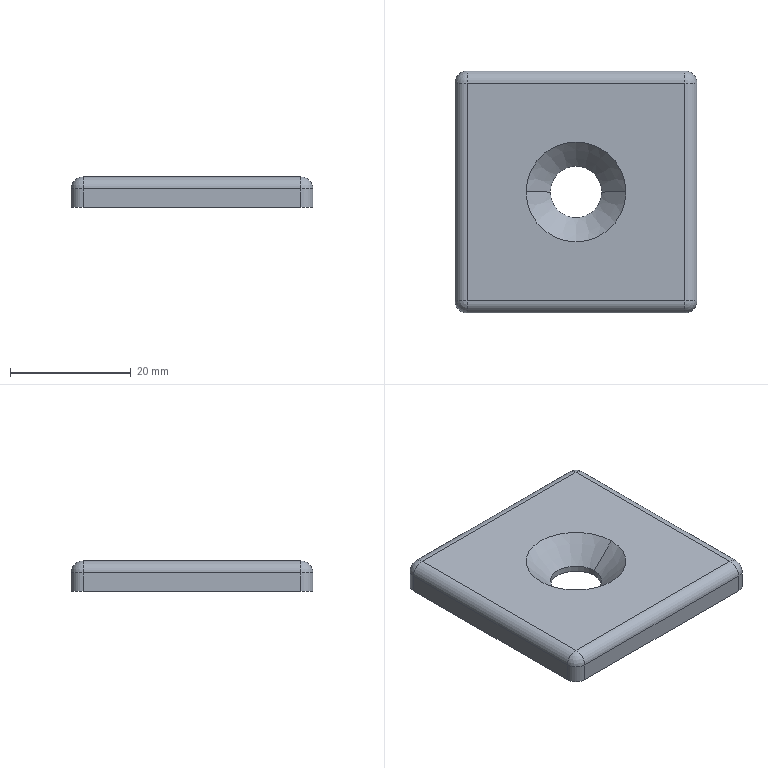Part | NX | features BREP 1 | 1 solid | 22 faces | box 40 x 40 x 5 mm | volume 7286 mm3 | cylinder 10 | plane 6 | sphere 4 | cone 2 | commonest cylinder face diameters 4 x8 8.5 x2
STEP:
#1=CARTESIAN_POINT('',(-4.25,0.,1.));
#2=VERTEX_POINT('',#1);
#3=CARTESIAN_POINT('',(4.25,0.,1.));
#4=VERTEX_POINT('',#3);
#5=CARTESIAN_POINT('',(0.,0.,1.));
#6=DIRECTION('',(0.,0.,1.));
#7=DIRECTION('',(-1.,0.,0.));
#8=AXIS2_PLACEMENT_3D('',#5,#6,#7);
#9=CIRCLE('',#8,4.25);
#10=EDGE_CURVE('',#2,#4,#9,.T.);
#11=ORIENTED_EDGE('',*,*,#10,.F.);
#12=CARTESIAN_POINT('',(-8.25,0.,5.));
#13=VERTEX_POINT('',#12);
#14=CARTESIAN_POINT('',(-4.25,0.,1.));
#15=DIRECTION('',(-0.7071,0.,0.7071));
#16=VECTOR('',#15,1000.);
#17=LINE('',#14,#16);
#18=EDGE_CURVE('',#13,#2,#17,.F.);
#19=ORIENTED_EDGE('',*,*,#18,.F.);
#20=CARTESIAN_POINT('',(8.25,0.,5.));
#21=VERTEX_POINT('',#20);
#22=CARTESIAN_POINT('',(0.,0.,5.));
#23=DIRECTION('',(0.,0.,-1.));
#24=DIRECTION('',(-1.,0.,0.));
#25=AXIS2_PLACEMENT_3D('',#22,#23,#24);
#26=CIRCLE('',#25,8.25);
#27=EDGE_CURVE('',#21,#13,#26,.T.);
#28=ORIENTED_EDGE('',*,*,#27,.F.);
#29=CARTESIAN_POINT('',(4.25,0.,1.));
#30=DIRECTION('',(0.7071,0.,0.7071));
#31=VECTOR('',#30,1000.);
#32=LINE('',#29,#31);
#33=EDGE_CURVE('',#21,#4,#32,.F.);
#34=ORIENTED_EDGE('',*,*,#33,.T.);
#35=EDGE_LOOP('',(#11,#19,#28,#34));
#36=FACE_BOUND('',#35,.T.);
#37=CARTESIAN_POINT('',(0.,0.,1.));
#38=DIRECTION('',(0.,0.,1.));
#39=DIRECTION('',(1.,0.,0.));
#40=AXIS2_PLACEMENT_3D('',#37,#38,#39);
#41=CONICAL_SURFACE('',#40,4.25,0.7854);
#42=ADVANCED_FACE('',(#36),#41,.F.);
#43=CARTESIAN_POINT('',(-4.25,0.,0.));
#44=VERTEX_POINT('',#43);
#45=CARTESIAN_POINT('',(4.25,0.,0.));
#46=VERTEX_POINT('',#45);
#47=CARTESIAN_POINT('',(0.,0.,0.));
#48=DIRECTION('',(0.,0.,1.));
#49=DIRECTION('',(1.,0.,0.));
#50=AXIS2_PLACEMENT_3D('',#47,#48,#49);
#51=CIRCLE('',#50,4.25);
#52=EDGE_CURVE('',#44,#46,#51,.T.);
#53=ORIENTED_EDGE('',*,*,#52,.F.);
#54=CARTESIAN_POINT('',(-4.25,0.,0.));
#55=DIRECTION('',(0.,0.,1.));
#56=VECTOR('',#55,1000.);
#57=LINE('',#54,#56);
#58=EDGE_CURVE('',#2,#44,#57,.F.);
#59=ORIENTED_EDGE('',*,*,#58,.F.);
#60=ORIENTED_EDGE('',*,*,#10,.T.);
#61=CARTESIAN_POINT('',(4.25,0.,0.));
#62=DIRECTION('',(0.,0.,1.));
#63=VECTOR('',#62,1000.);
#64=LINE('',#61,#63);
#65=EDGE_CURVE('',#4,#46,#64,.F.);
#66=ORIENTED_EDGE('',*,*,#65,.T.);
#67=EDGE_LOOP('',(#53,#59,#60,#66));
#68=FACE_BOUND('',#67,.T.);
#69=CARTESIAN_POINT('',(0.,0.,0.));
#70=DIRECTION('',(0.,0.,1.));
#71=DIRECTION('',(1.,0.,0.));
#72=AXIS2_PLACEMENT_3D('',#69,#70,#71);
#73=CYLINDRICAL_SURFACE('',#72,4.25);
#74=ADVANCED_FACE('',(#68),#73,.F.);
#75=CARTESIAN_POINT('',(20.,-18.,0.));
#76=VERTEX_POINT('',#75);
#77=CARTESIAN_POINT('',(20.,18.,0.));
#78=VERTEX_POINT('',#77);
#79=CARTESIAN_POINT('',(20.,-20.,0.));
#80=DIRECTION('',(0.,1.,0.));
#81=VECTOR('',#80,1000.);
#82=LINE('',#79,#81);
#83=EDGE_CURVE('',#76,#78,#82,.T.);
#84=ORIENTED_EDGE('',*,*,#83,.T.);
#85=CARTESIAN_POINT('',(20.,18.,3.));
#86=VERTEX_POINT('',#85);
#87=CARTESIAN_POINT('',(20.,18.,5.));
#88=DIRECTION('',(0.,0.,1.));
#89=VECTOR('',#88,1000.);
#90=LINE('',#87,#89);
#91=EDGE_CURVE('',#78,#86,#90,.T.);
#92=ORIENTED_EDGE('',*,*,#91,.T.);
#93=CARTESIAN_POINT('',(20.,-18.,3.));
#94=VERTEX_POINT('',#93);
#95=CARTESIAN_POINT('',(20.,-20.,3.));
#96=DIRECTION('',(0.,-1.,0.));
#97=VECTOR('',#96,1000.);
#98=LINE('',#95,#97);
#99=EDGE_CURVE('',#86,#94,#98,.T.);
#100=ORIENTED_EDGE('',*,*,#99,.T.);
#101=CARTESIAN_POINT('',(20.,-18.,5.));
#102=DIRECTION('',(0.,0.,-1.));
#103=VECTOR('',#102,1000.);
#104=LINE('',#101,#103);
#105=EDGE_CURVE('',#94,#76,#104,.T.);
#106=ORIENTED_EDGE('',*,*,#105,.T.);
#107=EDGE_LOOP('',(#84,#92,#100,#106));
#108=FACE_BOUND('',#107,.T.);
#109=CARTESIAN_POINT('',(20.,-20.,5.));
#110=DIRECTION('',(-1.,0.,0.));
#111=DIRECTION('',(0.,0.,1.));
#112=AXIS2_PLACEMENT_3D('',#109,#110,#111);
#113=PLANE('',#112);
#114=ADVANCED_FACE('',(#108),#113,.F.);
#115=CARTESIAN_POINT('',(18.,20.,0.));
#116=VERTEX_POINT('',#115);
#117=CARTESIAN_POINT('',(-18.,20.,0.));
#118=VERTEX_POINT('',#117);
#119=CARTESIAN_POINT('',(-20.,20.,0.));
#120=DIRECTION('',(-1.,0.,0.));
#121=VECTOR('',#120,1000.);
#122=LINE('',#119,#121);
#123=EDGE_CURVE('',#116,#118,#122,.T.);
#124=ORIENTED_EDGE('',*,*,#123,.T.);
#125=CARTESIAN_POINT('',(-18.,20.,3.));
#126=VERTEX_POINT('',#125);
#127=CARTESIAN_POINT('',(-18.,20.,5.));
#128=DIRECTION('',(0.,0.,1.));
#129=VECTOR('',#128,1000.);
#130=LINE('',#127,#129);
#131=EDGE_CURVE('',#118,#126,#130,.T.);
#132=ORIENTED_EDGE('',*,*,#131,.T.);
#133=CARTESIAN_POINT('',(18.,20.,3.));
#134=VERTEX_POINT('',#133);
#135=CARTESIAN_POINT('',(-20.,20.,3.));
#136=DIRECTION('',(1.,0.,0.));
#137=VECTOR('',#136,1000.);
#138=LINE('',#135,#137);
#139=EDGE_CURVE('',#126,#134,#138,.T.);
#140=ORIENTED_EDGE('',*,*,#139,.T.);
#141=CARTESIAN_POINT('',(18.,20.,5.));
#142=DIRECTION('',(0.,0.,-1.));
#143=VECTOR('',#142,1000.);
#144=LINE('',#141,#143);
#145=EDGE_CURVE('',#134,#116,#144,.T.);
#146=ORIENTED_EDGE('',*,*,#145,.T.);
#147=EDGE_LOOP('',(#124,#132,#140,#146));
#148=FACE_BOUND('',#147,.T.);
#149=CARTESIAN_POINT('',(-20.,20.,5.));
#150=DIRECTION('',(0.,-1.,0.));
#151=DIRECTION('',(0.,0.,-1.));
#152=AXIS2_PLACEMENT_3D('',#149,#150,#151);
#153=PLANE('',#152);
#154=ADVANCED_FACE('',(#148),#153,.F.);
#155=CARTESIAN_POINT('',(-20.,-18.,3.));
#156=VERTEX_POINT('',#155);
#157=CARTESIAN_POINT('',(-20.,18.,3.));
#158=VERTEX_POINT('',#157);
#159=CARTESIAN_POINT('',(-20.,-20.,3.));
#160=DIRECTION('',(0.,1.,0.));
#161=VECTOR('',#160,1000.);
#162=LINE('',#159,#161);
#163=EDGE_CURVE('',#156,#158,#162,.T.);
#164=ORIENTED_EDGE('',*,*,#163,.T.);
#165=CARTESIAN_POINT('',(-20.,18.,0.));
#166=VERTEX_POINT('',#165);
#167=CARTESIAN_POINT('',(-20.,18.,5.));
#168=DIRECTION('',(0.,0.,-1.));
#169=VECTOR('',#168,1000.);
#170=LINE('',#167,#169);
#171=EDGE_CURVE('',#158,#166,#170,.T.);
#172=ORIENTED_EDGE('',*,*,#171,.T.);
#173=CARTESIAN_POINT('',(-20.,-18.,0.));
#174=VERTEX_POINT('',#173);
#175=CARTESIAN_POINT('',(-20.,-20.,0.));
#176=DIRECTION('',(0.,-1.,0.));
#177=VECTOR('',#176,1000.);
#178=LINE('',#175,#177);
#179=EDGE_CURVE('',#166,#174,#178,.T.);
#180=ORIENTED_EDGE('',*,*,#179,.T.);
#181=CARTESIAN_POINT('',(-20.,-18.,5.));
#182=DIRECTION('',(0.,0.,1.));
#183=VECTOR('',#182,1000.);
#184=LINE('',#181,#183);
#185=EDGE_CURVE('',#174,#156,#184,.T.);
#186=ORIENTED_EDGE('',*,*,#185,.T.);
#187=EDGE_LOOP('',(#164,#172,#180,#186));
#188=FACE_BOUND('',#187,.T.);
#189=CARTESIAN_POINT('',(-20.,-20.,5.));
#190=DIRECTION('',(1.,0.,0.));
#191=DIRECTION('',(0.,1.,0.));
#192=AXIS2_PLACEMENT_3D('',#189,#190,#191);
#193=PLANE('',#192);
#194=ADVANCED_FACE('',(#188),#193,.F.);
#195=CARTESIAN_POINT('',(-18.,-20.,0.));
#196=VERTEX_POINT('',#195);
#197=CARTESIAN_POINT('',(18.,-20.,0.));
#198=VERTEX_POINT('',#197);
#199=CARTESIAN_POINT('',(-20.,-20.,0.));
#200=DIRECTION('',(1.,0.,0.));
#201=VECTOR('',#200,1000.);
#202=LINE('',#199,#201);
#203=EDGE_CURVE('',#196,#198,#202,.T.);
#204=ORIENTED_EDGE('',*,*,#203,.T.);
#205=CARTESIAN_POINT('',(18.,-20.,3.));
#206=VERTEX_POINT('',#205);
#207=CARTESIAN_POINT('',(18.,-20.,5.));
#208=DIRECTION('',(0.,0.,1.));
#209=VECTOR('',#208,1000.);
#210=LINE('',#207,#209);
#211=EDGE_CURVE('',#198,#206,#210,.T.);
#212=ORIENTED_EDGE('',*,*,#211,.T.);
#213=CARTESIAN_POINT('',(-18.,-20.,3.));
#214=VERTEX_POINT('',#213);
#215=CARTESIAN_POINT('',(-20.,-20.,3.));
#216=DIRECTION('',(-1.,0.,0.));
#217=VECTOR('',#216,1000.);
#218=LINE('',#215,#217);
#219=EDGE_CURVE('',#206,#214,#218,.T.);
#220=ORIENTED_EDGE('',*,*,#219,.T.);
#221=CARTESIAN_POINT('',(-18.,-20.,5.));
#222=DIRECTION('',(0.,0.,-1.));
#223=VECTOR('',#222,1000.);
#224=LINE('',#221,#223);
#225=EDGE_CURVE('',#214,#196,#224,.T.);
#226=ORIENTED_EDGE('',*,*,#225,.T.);
#227=EDGE_LOOP('',(#204,#212,#220,#226));
#228=FACE_BOUND('',#227,.T.);
#229=CARTESIAN_POINT('',(-20.,-20.,5.));
#230=DIRECTION('',(0.,1.,0.));
#231=DIRECTION('',(1.,0.,0.));
#232=AXIS2_PLACEMENT_3D('',#229,#230,#231);
#233=PLANE('',#232);
#234=ADVANCED_FACE('',(#228),#233,.F.);
#235=CARTESIAN_POINT('',(-18.,18.,5.));
#236=VERTEX_POINT('',#235);
#237=CARTESIAN_POINT('',(-18.,-18.,5.));
#238=VERTEX_POINT('',#237);
#239=CARTESIAN_POINT('',(-18.,0.,5.));
#240=DIRECTION('',(0.,-1.,0.));
#241=VECTOR('',#240,1000.);
#242=LINE('',#239,#241);
#243=EDGE_CURVE('',#236,#238,#242,.T.);
#244=ORIENTED_EDGE('',*,*,#243,.T.);
#245=CARTESIAN_POINT('',(18.,-18.,5.));
#246=VERTEX_POINT('',#245);
#247=CARTESIAN_POINT('',(0.,-18.,5.));
#248=DIRECTION('',(1.,0.,0.));
#249=VECTOR('',#248,1000.);
#250=LINE('',#247,#249);
#251=EDGE_CURVE('',#238,#246,#250,.T.);
#252=ORIENTED_EDGE('',*,*,#251,.T.);
#253=CARTESIAN_POINT('',(18.,18.,5.));
#254=VERTEX_POINT('',#253);
#255=CARTESIAN_POINT('',(18.,0.,5.));
#256=DIRECTION('',(0.,1.,0.));
#257=VECTOR('',#256,1000.);
#258=LINE('',#255,#257);
#259=EDGE_CURVE('',#246,#254,#258,.T.);
#260=ORIENTED_EDGE('',*,*,#259,.T.);
#261=CARTESIAN_POINT('',(0.,18.,5.));
#262=DIRECTION('',(-1.,0.,0.));
#263=VECTOR('',#262,1000.);
#264=LINE('',#261,#263);
#265=EDGE_CURVE('',#254,#236,#264,.T.);
#266=ORIENTED_EDGE('',*,*,#265,.T.);
#267=EDGE_LOOP('',(#244,#252,#260,#266));
#268=FACE_BOUND('',#267,.T.);
#269=ORIENTED_EDGE('',*,*,#27,.T.);
#270=CARTESIAN_POINT('',(0.,0.,5.));
#271=DIRECTION('',(0.,0.,-1.));
#272=DIRECTION('',(-1.,0.,0.));
#273=AXIS2_PLACEMENT_3D('',#270,#271,#272);
#274=CIRCLE('',#273,8.25);
#275=EDGE_CURVE('',#13,#21,#274,.T.);
#276=ORIENTED_EDGE('',*,*,#275,.T.);
#277=EDGE_LOOP('',(#269,#276));
#278=FACE_BOUND('',#277,.T.);
#279=CARTESIAN_POINT('',(0.,0.,5.));
#280=DIRECTION('',(0.,0.,-1.));
#281=DIRECTION('',(0.,-1.,0.));
#282=AXIS2_PLACEMENT_3D('',#279,#280,#281);
#283=PLANE('',#282);
#284=ADVANCED_FACE('',(#268,#278),#283,.F.);
#285=ORIENTED_EDGE('',*,*,#179,.F.);
#286=CARTESIAN_POINT('',(-18.,18.,0.));
#287=DIRECTION('',(0.,0.,-1.));
#288=DIRECTION('',(-1.,0.,0.));
#289=AXIS2_PLACEMENT_3D('',#286,#287,#288);
#290=CIRCLE('',#289,2.);
#291=EDGE_CURVE('',#166,#118,#290,.T.);
#292=ORIENTED_EDGE('',*,*,#291,.T.);
#293=ORIENTED_EDGE('',*,*,#123,.F.);
#294=CARTESIAN_POINT('',(18.,18.,0.));
#295=DIRECTION('',(0.,0.,-1.));
#296=DIRECTION('',(-1.,0.,0.));
#297=AXIS2_PLACEMENT_3D('',#294,#295,#296);
#298=CIRCLE('',#297,2.);
#299=EDGE_CURVE('',#116,#78,#298,.T.);
#300=ORIENTED_EDGE('',*,*,#299,.T.);
#301=ORIENTED_EDGE('',*,*,#83,.F.);
#302=CARTESIAN_POINT('',(18.,-18.,0.));
#303=DIRECTION('',(0.,0.,-1.));
#304=DIRECTION('',(-1.,0.,0.));
#305=AXIS2_PLACEMENT_3D('',#302,#303,#304);
#306=CIRCLE('',#305,2.);
#307=EDGE_CURVE('',#76,#198,#306,.T.);
#308=ORIENTED_EDGE('',*,*,#307,.T.);
#309=ORIENTED_EDGE('',*,*,#203,.F.);
#310=CARTESIAN_POINT('',(-18.,-18.,0.));
#311=DIRECTION('',(0.,0.,-1.));
#312=DIRECTION('',(-1.,0.,0.));
#313=AXIS2_PLACEMENT_3D('',#310,#311,#312);
#314=CIRCLE('',#313,2.);
#315=EDGE_CURVE('',#196,#174,#314,.T.);
#316=ORIENTED_EDGE('',*,*,#315,.T.);
#317=EDGE_LOOP('',(#285,#292,#293,#300,#301,#308,#309,#316));
#318=FACE_BOUND('',#317,.T.);
#319=CARTESIAN_POINT('',(0.,0.,0.));
#320=DIRECTION('',(0.,0.,1.));
#321=DIRECTION('',(1.,0.,0.));
#322=AXIS2_PLACEMENT_3D('',#319,#320,#321);
#323=CIRCLE('',#322,4.25);
#324=EDGE_CURVE('',#46,#44,#323,.T.);
#325=ORIENTED_EDGE('',*,*,#324,.T.);
#326=ORIENTED_EDGE('',*,*,#52,.T.);
#327=EDGE_LOOP('',(#325,#326));
#328=FACE_BOUND('',#327,.T.);
#329=CARTESIAN_POINT('',(0.,0.,0.));
#330=DIRECTION('',(0.,0.,-1.));
#331=DIRECTION('',(0.,-1.,0.));
#332=AXIS2_PLACEMENT_3D('',#329,#330,#331);
#333=PLANE('',#332);
#334=ADVANCED_FACE('',(#318,#328),#333,.T.);
#335=ORIENTED_EDGE('',*,*,#291,.F.);
#336=ORIENTED_EDGE('',*,*,#171,.F.);
#337=CARTESIAN_POINT('',(-18.,18.,3.));
#338=DIRECTION('',(0.,0.,1.));
#339=DIRECTION('',(1.,0.,0.));
#340=AXIS2_PLACEMENT_3D('',#337,#338,#339);
#341=CIRCLE('',#340,2.);
#342=EDGE_CURVE('',#126,#158,#341,.T.);
#343=ORIENTED_EDGE('',*,*,#342,.F.);
#344=ORIENTED_EDGE('',*,*,#131,.F.);
#345=EDGE_LOOP('',(#335,#336,#343,#344));
#346=FACE_BOUND('',#345,.T.);
#347=CARTESIAN_POINT('',(-18.,18.,5.));
#348=DIRECTION('',(0.,0.,-1.));
#349=DIRECTION('',(-1.,0.,0.));
#350=AXIS2_PLACEMENT_3D('',#347,#348,#349);
#351=CYLINDRICAL_SURFACE('',#350,2.);
#352=ADVANCED_FACE('',(#346),#351,.T.);
#353=CARTESIAN_POINT('',(18.,18.,3.));
#354=DIRECTION('',(1.,0.,0.));
#355=DIRECTION('',(0.,0.,-1.));
#356=AXIS2_PLACEMENT_3D('',#353,#354,#355);
#357=CIRCLE('',#356,2.);
#358=EDGE_CURVE('',#134,#254,#357,.T.);
#359=ORIENTED_EDGE('',*,*,#358,.F.);
#360=ORIENTED_EDGE('',*,*,#139,.F.);
#361=CARTESIAN_POINT('',(-18.,18.,3.));
#362=DIRECTION('',(-1.,0.,0.));
#363=DIRECTION('',(0.,0.,1.));
#364=AXIS2_PLACEMENT_3D('',#361,#362,#363);
#365=CIRCLE('',#364,2.);
#366=EDGE_CURVE('',#236,#126,#365,.T.);
#367=ORIENTED_EDGE('',*,*,#366,.F.);
#368=ORIENTED_EDGE('',*,*,#265,.F.);
#369=EDGE_LOOP('',(#359,#360,#367,#368));
#370=FACE_BOUND('',#369,.T.);
#371=CARTESIAN_POINT('',(0.,18.,3.));
#372=DIRECTION('',(-1.,0.,0.));
#373=DIRECTION('',(0.,0.,1.));
#374=AXIS2_PLACEMENT_3D('',#371,#372,#373);
#375=CYLINDRICAL_SURFACE('',#374,2.);
#376=ADVANCED_FACE('',(#370),#375,.T.);
#377=ORIENTED_EDGE('',*,*,#299,.F.);
#378=ORIENTED_EDGE('',*,*,#145,.F.);
#379=CARTESIAN_POINT('',(18.,18.,3.));
#380=DIRECTION('',(0.,0.,1.));
#381=DIRECTION('',(1.,0.,0.));
#382=AXIS2_PLACEMENT_3D('',#379,#380,#381);
#383=CIRCLE('',#382,2.);
#384=EDGE_CURVE('',#86,#134,#383,.T.);
#385=ORIENTED_EDGE('',*,*,#384,.F.);
#386=ORIENTED_EDGE('',*,*,#91,.F.);
#387=EDGE_LOOP('',(#377,#378,#385,#386));
#388=FACE_BOUND('',#387,.T.);
#389=CARTESIAN_POINT('',(18.,18.,5.));
#390=DIRECTION('',(0.,0.,-1.));
#391=DIRECTION('',(-1.,0.,0.));
#392=AXIS2_PLACEMENT_3D('',#389,#390,#391);
#393=CYLINDRICAL_SURFACE('',#392,2.);
#394=ADVANCED_FACE('',(#388),#393,.T.);
#395=ORIENTED_EDGE('',*,*,#366,.T.);
#396=ORIENTED_EDGE('',*,*,#342,.T.);
#397=CARTESIAN_POINT('',(-18.,18.,3.));
#398=DIRECTION('',(0.,-1.,0.));
#399=DIRECTION('',(0.,0.,1.));
#400=AXIS2_PLACEMENT_3D('',#397,#398,#399);
#401=CIRCLE('',#400,2.);
#402=EDGE_CURVE('',#236,#158,#401,.T.);
#403=ORIENTED_EDGE('',*,*,#402,.F.);
#404=EDGE_LOOP('',(#395,#396,#403));
#405=FACE_BOUND('',#404,.T.);
#406=CARTESIAN_POINT('',(-18.,18.,3.));
#407=DIRECTION('',(0.,0.,-1.));
#408=DIRECTION('',(1.,0.,0.));
#409=AXIS2_PLACEMENT_3D('',#406,#407,#408);
#410=SPHERICAL_SURFACE('',#409,2.);
#411=ADVANCED_FACE('',(#405),#410,.T.);
#412=ORIENTED_EDGE('',*,*,#384,.T.);
#413=ORIENTED_EDGE('',*,*,#358,.T.);
#414=CARTESIAN_POINT('',(18.,18.,3.));
#415=DIRECTION('',(0.,-1.,0.));
#416=DIRECTION('',(0.,0.,1.));
#417=AXIS2_PLACEMENT_3D('',#414,#415,#416);
#418=CIRCLE('',#417,2.);
#419=EDGE_CURVE('',#86,#254,#418,.T.);
#420=ORIENTED_EDGE('',*,*,#419,.F.);
#421=EDGE_LOOP('',(#412,#413,#420));
#422=FACE_BOUND('',#421,.T.);
#423=CARTESIAN_POINT('',(18.,18.,3.));
#424=DIRECTION('',(0.,0.,-1.));
#425=DIRECTION('',(1.,0.,0.));
#426=AXIS2_PLACEMENT_3D('',#423,#424,#425);
#427=SPHERICAL_SURFACE('',#426,2.);
#428=ADVANCED_FACE('',(#422),#427,.T.);
#429=ORIENTED_EDGE('',*,*,#315,.F.);
#430=ORIENTED_EDGE('',*,*,#225,.F.);
#431=CARTESIAN_POINT('',(-18.,-18.,3.));
#432=DIRECTION('',(0.,0.,1.));
#433=DIRECTION('',(1.,0.,0.));
#434=AXIS2_PLACEMENT_3D('',#431,#432,#433);
#435=CIRCLE('',#434,2.);
#436=EDGE_CURVE('',#156,#214,#435,.T.);
#437=ORIENTED_EDGE('',*,*,#436,.F.);
#438=ORIENTED_EDGE('',*,*,#185,.F.);
#439=EDGE_LOOP('',(#429,#430,#437,#438));
#440=FACE_BOUND('',#439,.T.);
#441=CARTESIAN_POINT('',(-18.,-18.,5.));
#442=DIRECTION('',(0.,0.,-1.));
#443=DIRECTION('',(-1.,0.,0.));
#444=AXIS2_PLACEMENT_3D('',#441,#442,#443);
#445=CYLINDRICAL_SURFACE('',#444,2.);
#446=ADVANCED_FACE('',(#440),#445,.T.);
#447=ORIENTED_EDGE('',*,*,#402,.T.);
#448=ORIENTED_EDGE('',*,*,#163,.F.);
#449=CARTESIAN_POINT('',(-18.,-18.,3.));
#450=DIRECTION('',(0.,-1.,0.));
#451=DIRECTION('',(0.,0.,-1.));
#452=AXIS2_PLACEMENT_3D('',#449,#450,#451);
#453=CIRCLE('',#452,2.);
#454=EDGE_CURVE('',#238,#156,#453,.T.);
#455=ORIENTED_EDGE('',*,*,#454,.F.);
#456=ORIENTED_EDGE('',*,*,#243,.F.);
#457=EDGE_LOOP('',(#447,#448,#455,#456));
#458=FACE_BOUND('',#457,.T.);
#459=CARTESIAN_POINT('',(-18.,0.,3.));
#460=DIRECTION('',(0.,-1.,0.));
#461=DIRECTION('',(0.,0.,-1.));
#462=AXIS2_PLACEMENT_3D('',#459,#460,#461);
#463=CYLINDRICAL_SURFACE('',#462,2.);
#464=ADVANCED_FACE('',(#458),#463,.T.);
#465=ORIENTED_EDGE('',*,*,#419,.T.);
#466=ORIENTED_EDGE('',*,*,#259,.F.);
#467=CARTESIAN_POINT('',(18.,-18.,3.));
#468=DIRECTION('',(0.,-1.,0.));
#469=DIRECTION('',(0.,0.,-1.));
#470=AXIS2_PLACEMENT_3D('',#467,#468,#469);
#471=CIRCLE('',#470,2.);
#472=EDGE_CURVE('',#94,#246,#471,.T.);
#473=ORIENTED_EDGE('',*,*,#472,.F.);
#474=ORIENTED_EDGE('',*,*,#99,.F.);
#475=EDGE_LOOP('',(#465,#466,#473,#474));
#476=FACE_BOUND('',#475,.T.);
#477=CARTESIAN_POINT('',(18.,0.,3.));
#478=DIRECTION('',(0.,1.,0.));
#479=DIRECTION('',(0.,0.,1.));
#480=AXIS2_PLACEMENT_3D('',#477,#478,#479);
#481=CYLINDRICAL_SURFACE('',#480,2.);
#482=ADVANCED_FACE('',(#476),#481,.T.);
#483=ORIENTED_EDGE('',*,*,#307,.F.);
#484=ORIENTED_EDGE('',*,*,#105,.F.);
#485=CARTESIAN_POINT('',(18.,-18.,3.));
#486=DIRECTION('',(0.,0.,1.));
#487=DIRECTION('',(1.,0.,0.));
#488=AXIS2_PLACEMENT_3D('',#485,#486,#487);
#489=CIRCLE('',#488,2.);
#490=EDGE_CURVE('',#206,#94,#489,.T.);
#491=ORIENTED_EDGE('',*,*,#490,.F.);
#492=ORIENTED_EDGE('',*,*,#211,.F.);
#493=EDGE_LOOP('',(#483,#484,#491,#492));
#494=FACE_BOUND('',#493,.T.);
#495=CARTESIAN_POINT('',(18.,-18.,5.));
#496=DIRECTION('',(0.,0.,-1.));
#497=DIRECTION('',(-1.,0.,0.));
#498=AXIS2_PLACEMENT_3D('',#495,#496,#497);
#499=CYLINDRICAL_SURFACE('',#498,2.);
#500=ADVANCED_FACE('',(#494),#499,.T.);
#501=ORIENTED_EDGE('',*,*,#454,.T.);
#502=ORIENTED_EDGE('',*,*,#436,.T.);
#503=CARTESIAN_POINT('',(-18.,-18.,3.));
#504=DIRECTION('',(1.,0.,0.));
#505=DIRECTION('',(0.,0.,1.));
#506=AXIS2_PLACEMENT_3D('',#503,#504,#505);
#507=CIRCLE('',#506,2.);
#508=EDGE_CURVE('',#238,#214,#507,.T.);
#509=ORIENTED_EDGE('',*,*,#508,.F.);
#510=EDGE_LOOP('',(#501,#502,#509));
#511=FACE_BOUND('',#510,.T.);
#512=CARTESIAN_POINT('',(-18.,-18.,3.));
#513=DIRECTION('',(0.,0.,-1.));
#514=DIRECTION('',(1.,0.,0.));
#515=AXIS2_PLACEMENT_3D('',#512,#513,#514);
#516=SPHERICAL_SURFACE('',#515,2.);
#517=ADVANCED_FACE('',(#511),#516,.T.);
#518=ORIENTED_EDGE('',*,*,#490,.T.);
#519=ORIENTED_EDGE('',*,*,#472,.T.);
#520=CARTESIAN_POINT('',(18.,-18.,3.));
#521=DIRECTION('',(-1.,0.,0.));
#522=DIRECTION('',(0.,0.,-1.));
#523=AXIS2_PLACEMENT_3D('',#520,#521,#522);
#524=CIRCLE('',#523,2.);
#525=EDGE_CURVE('',#206,#246,#524,.T.);
#526=ORIENTED_EDGE('',*,*,#525,.F.);
#527=EDGE_LOOP('',(#518,#519,#526));
#528=FACE_BOUND('',#527,.T.);
#529=CARTESIAN_POINT('',(18.,-18.,3.));
#530=DIRECTION('',(0.,0.,-1.));
#531=DIRECTION('',(1.,0.,0.));
#532=AXIS2_PLACEMENT_3D('',#529,#530,#531);
#533=SPHERICAL_SURFACE('',#532,2.);
#534=ADVANCED_FACE('',(#528),#533,.T.);
#535=ORIENTED_EDGE('',*,*,#508,.T.);
#536=ORIENTED_EDGE('',*,*,#219,.F.);
#537=ORIENTED_EDGE('',*,*,#525,.T.);
#538=ORIENTED_EDGE('',*,*,#251,.F.);
#539=EDGE_LOOP('',(#535,#536,#537,#538));
#540=FACE_BOUND('',#539,.T.);
#541=CARTESIAN_POINT('',(0.,-18.,3.));
#542=DIRECTION('',(1.,0.,0.));
#543=DIRECTION('',(0.,0.,-1.));
#544=AXIS2_PLACEMENT_3D('',#541,#542,#543);
#545=CYLINDRICAL_SURFACE('',#544,2.);
#546=ADVANCED_FACE('',(#540),#545,.T.);
#547=ORIENTED_EDGE('',*,*,#58,.T.);
#548=ORIENTED_EDGE('',*,*,#324,.F.);
#549=ORIENTED_EDGE('',*,*,#65,.F.);
#550=CARTESIAN_POINT('',(0.,0.,1.));
#551=DIRECTION('',(0.,0.,1.));
#552=DIRECTION('',(-1.,0.,0.));
#553=AXIS2_PLACEMENT_3D('',#550,#551,#552);
#554=CIRCLE('',#553,4.25);
#555=EDGE_CURVE('',#4,#2,#554,.T.);
#556=ORIENTED_EDGE('',*,*,#555,.T.);
#557=EDGE_LOOP('',(#547,#548,#549,#556));
#558=FACE_BOUND('',#557,.T.);
#559=CARTESIAN_POINT('',(0.,0.,0.));
#560=DIRECTION('',(0.,0.,1.));
#561=DIRECTION('',(1.,0.,0.));
#562=AXIS2_PLACEMENT_3D('',#559,#560,#561);
#563=CYLINDRICAL_SURFACE('',#562,4.25);
#564=ADVANCED_FACE('',(#558),#563,.F.);
#565=ORIENTED_EDGE('',*,*,#18,.T.);
#566=ORIENTED_EDGE('',*,*,#555,.F.);
#567=ORIENTED_EDGE('',*,*,#33,.F.);
#568=ORIENTED_EDGE('',*,*,#275,.F.);
#569=EDGE_LOOP('',(#565,#566,#567,#568));
#570=FACE_BOUND('',#569,.T.);
#571=CARTESIAN_POINT('',(0.,0.,1.));
#572=DIRECTION('',(0.,0.,1.));
#573=DIRECTION('',(1.,0.,0.));
#574=AXIS2_PLACEMENT_3D('',#571,#572,#573);
#575=CONICAL_SURFACE('',#574,4.25,0.7854);
#576=ADVANCED_FACE('',(#570),#575,.F.);
#577=CLOSED_SHELL('',(#42,#74,#114,#154,#194,#234,#284,#334,#352,#376,#394,#411,#428,#446,#464,#482,#500,#517,#534,#546,#564,#576));
#578=MANIFOLD_SOLID_BREP('',#577);
#579=(LENGTH_UNIT()NAMED_UNIT(*)SI_UNIT(.MILLI.,.METRE.));
#580=UNCERTAINTY_MEASURE_WITH_UNIT(LENGTH_MEASURE(0.00001),#579,'','');
#581=(NAMED_UNIT(*)PLANE_ANGLE_UNIT()SI_UNIT($,.RADIAN.));
#582=(NAMED_UNIT(*)SI_UNIT($,.STERADIAN.)SOLID_ANGLE_UNIT());
#583=(GEOMETRIC_REPRESENTATION_CONTEXT(3)GLOBAL_UNCERTAINTY_ASSIGNED_CONTEXT((#580))GLOBAL_UNIT_ASSIGNED_CONTEXT((#579,#581,#582))REPRESENTATION_CONTEXT('',''));
#584=ADVANCED_BREP_SHAPE_REPRESENTATION('',(#578),#583);